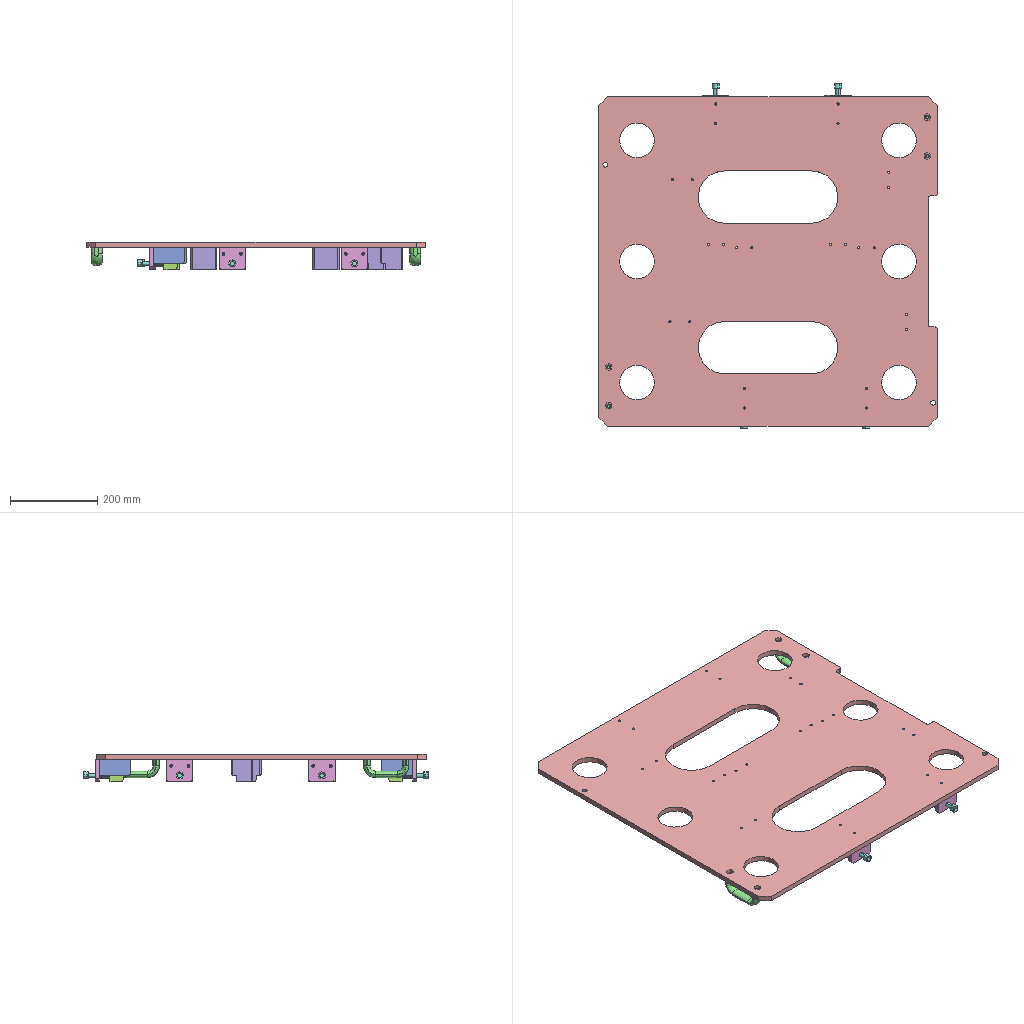Assembly | SolidWorks | 13 different items | 49 placed | box 775 x 789 x 64 mm
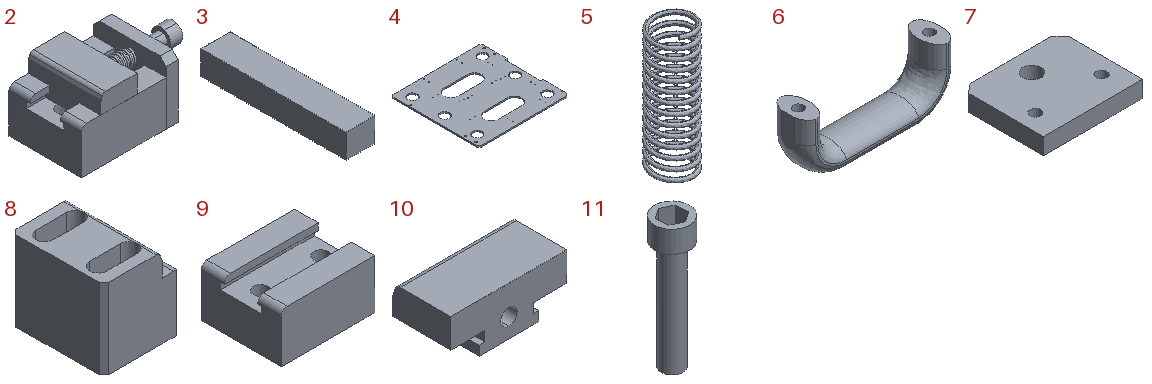Parts list (item | name | quantity | parent item | size | volume | features):
1 | (subassembly) | x1 | - | - | - | -
2 | (subassembly) | x6 | - | 106 x 60 x 52 mm | 199057 mm3 | -
3 | - | x1 | - | 12 x 60 x 10 mm | 7200 mm3 | features Extrusion 1
4 | - | x1 | - | 775 x 755 x 12 mm | 5715075 mm3 | features Cut 2, HoleWzd 2, ICE 2, Chamfer 1, Extrusion 1, Fillet 1
5 | - | x6 | in 2 | 13.2 x 13.2 x 41.299 mm | 661.875 mm3 | features ICE 2, Helix 1, Sweep 1
6 | - | x2 | - | 103 x 24.9 x 42.5 mm | 40167 mm3 | features CutThin 1, HoleWzd 1, Sweep 1
7 | - | x6 | in 2 | 60 x 50 x 10 mm | 28136 mm3 | features Cut 2, Chamfer 1, Extrusion 1
8 | - | x6 | - | 50 x 60 x 52 mm | 117515 mm3 | features ICE 3, Chamfer 2, Fillet 2, Extrusion 1
9 | - | x6 | in 2 | 70 x 60 x 37 mm | 131374 mm3 | features HoleWzd 2, Extrusion 1, Fillet 1, ICE 1
10 | - | x6 | in 2 | 60 x 30 x 25 mm | 33639 mm3 | features Chamfer 1, Cut 1, Extrusion 1, Fillet 1, HoleWzd 1, ICE 1
11 | - | x6 | in 2 | 16 x 16 x 60 mm | 5245 mm3 | features ICE 2, Extrusion 1
12 | W11300311 | x1 | - | - | - | -
13 | W11301705 | x1 | - | - | - | -
Mates (type | each side: item.copy, entity, surface, feature):
In the top assembly
Coincident | 4.1 face plane Boss-Extrude1 | 9.1 face plane Boss-Extrude1
Coincident | 4.1 face plane Boss-Extrude1 | 8.1 face plane Boss-Extrude1
Coincident | 4.1 face plane Boss-Extrude1 | 6.1 face plane Sweep1
DistanceDim | 4.1 face plane Boss-Extrude1 | 6.1 face plane Cut-Extrude-Thin1
DistanceDim | 6.1 face plane Cut-Extrude-Thin1 | 4.1 face plane Boss-Extrude1
Coincident | 4.1 face plane Boss-Extrude1 | 6.2 face plane Sweep1
DistanceDim | 6.2 face plane Cut-Extrude-Thin1 | 4.1 face plane Boss-Extrude1
DistanceDim | 4.1 face plane Boss-Extrude1 | 6.2 face plane Cut-Extrude-Thin1
Coincident | 4.1 face plane Boss-Extrude1 | 8.2 face plane Boss-Extrude1
Width | 8.2 face plane Boss-Extrude1 | 8.2 face plane Boss-Extrude1 | 9.1 face plane Boss-Extrude1 | 9.1 face plane Boss-Extrude1
Coincident | 4.1 face plane Boss-Extrude1 | 9.2 face plane Boss-Extrude1
DistanceDim | 4.1 face plane Boss-Extrude1 | 8.1 face plane Cut-Extrude1
DistanceDim | 4.1 face plane Boss-Extrude1 | 8.2 face plane Cut-Extrude1
Coincident | 4.1 face plane Boss-Extrude1 | 8.3 face plane Boss-Extrude1
DistanceDim | 4.1 face plane Boss-Extrude1 | 8.3 face plane Cut-Extrude1
Coincident | 8.3 face plane Boss-Extrude1 | 8.4 face plane Boss-Extrude1
DistanceDim | 8.2 face plane Boss-Extrude1 | 8.4 face plane Boss-Extrude1
DistanceDim | 8.4 face plane Cut-Extrude1 | 4.1 face plane Boss-Extrude1
DistanceDim | 9.1 face plane Boss-Extrude1 | 8.1 face plane Boss-Extrude1
Coincident | 4.1 face plane Boss-Extrude1 | 9.3 face plane Boss-Extrude1
Width | 9.3 face plane Boss-Extrude1 | 9.3 face plane Boss-Extrude1 | 8.4 face plane Boss-Extrude1 | 8.4 face plane Boss-Extrude1
Coincident | 10.1 face plane Boss-Extrude1 | 10.2 face plane Boss-Extrude1
Width | 9.4 face plane Boss-Extrude1 | 9.4 face plane Boss-Extrude1 | 8.3 face plane Boss-Extrude1 | 8.3 face plane Boss-Extrude1
In subassembly 2
Coincident | 9.5 face plane Cut-Extrude2 | 10.3 face plane Boss-Extrude1
Width | 9.5 face plane Cut-Extrude2 | 9.5 face plane Cut-Extrude2 | 10.3 face plane Boss-Extrude1 | 10.3 face plane Boss-Extrude1
Coincident | 9.5 face plane Boss-Extrude1 | 7.1 face plane Boss-Extrude1 | 3 times
Concentric | 10.3 face cylinder M10 Tapped Hole1 | 11.1 face cylinder Boss-Extrude1
Concentric | 11.1 face cylinder Boss-Extrude1 | 5.1 face cylinder Cut-Extrude1
Coincident | 7.1 face plane Boss-Extrude1 | 5.1 face plane Cut-Extrude2
Coincident | 10.3 face plane Boss-Extrude1 | 11.1 face plane Boss-Extrude1
DistanceDim | 10.3 face plane Boss-Extrude1 | 9.5 face plane Boss-Extrude1